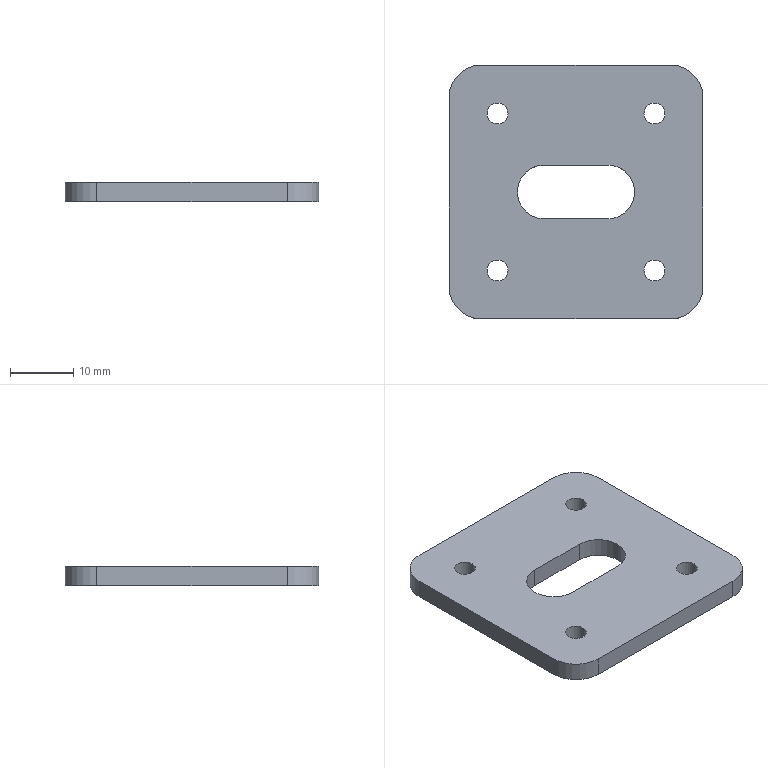Part | SolidWorks | features BaseBody 1 | 1 solid | 23 faces | box 40 x 40 x 3 mm | volume 4208 mm3 | cylinder 15 | plane 8 | commonest cylinder face diameters 3.3 x8 10 x4 8.5 x3
STEP:
#1=CARTESIAN_POINT('',(30.725,-32.375,0.));
#2=VERTEX_POINT('',#1);
#3=CARTESIAN_POINT('',(30.725,-32.375,3.));
#4=VERTEX_POINT('',#3);
#5=CARTESIAN_POINT('',(30.725,-32.375,3.));
#6=DIRECTION('',(0.,0.,1.));
#7=VECTOR('',#6,1000.);
#8=LINE('',#5,#7);
#9=EDGE_CURVE('',#2,#4,#8,.T.);
#10=ORIENTED_EDGE('',*,*,#9,.F.);
#11=CARTESIAN_POINT('',(34.025,-32.375,0.));
#12=VERTEX_POINT('',#11);
#13=CARTESIAN_POINT('',(32.375,-32.375,0.));
#14=DIRECTION('',(0.,0.,1.));
#15=DIRECTION('',(1.,0.,0.));
#16=AXIS2_PLACEMENT_3D('',#13,#14,#15);
#17=CIRCLE('',#16,1.65);
#18=EDGE_CURVE('',#12,#2,#17,.T.);
#19=ORIENTED_EDGE('',*,*,#18,.F.);
#20=CARTESIAN_POINT('',(34.025,-32.375,3.));
#21=VERTEX_POINT('',#20);
#22=CARTESIAN_POINT('',(34.025,-32.375,3.));
#23=DIRECTION('',(0.,0.,1.));
#24=VECTOR('',#23,1000.);
#25=LINE('',#22,#24);
#26=EDGE_CURVE('',#12,#21,#25,.T.);
#27=ORIENTED_EDGE('',*,*,#26,.T.);
#28=CARTESIAN_POINT('',(32.375,-32.375,3.));
#29=DIRECTION('',(0.,0.,1.));
#30=DIRECTION('',(1.,0.,0.));
#31=AXIS2_PLACEMENT_3D('',#28,#29,#30);
#32=CIRCLE('',#31,1.65);
#33=EDGE_CURVE('',#21,#4,#32,.T.);
#34=ORIENTED_EDGE('',*,*,#33,.T.);
#35=EDGE_LOOP('',(#10,#19,#27,#34));
#36=FACE_OUTER_BOUND('',#35,.T.);
#37=CARTESIAN_POINT('',(32.375,-32.375,3.));
#38=DIRECTION('',(0.,0.,1.));
#39=DIRECTION('',(1.,0.,0.));
#40=AXIS2_PLACEMENT_3D('',#37,#38,#39);
#41=CYLINDRICAL_SURFACE('',#40,1.65);
#42=ADVANCED_FACE('',(#36),#41,.F.);
#43=CARTESIAN_POINT('',(5.975,-32.375,0.));
#44=VERTEX_POINT('',#43);
#45=CARTESIAN_POINT('',(5.975,-32.375,3.));
#46=VERTEX_POINT('',#45);
#47=CARTESIAN_POINT('',(5.975,-32.375,3.));
#48=DIRECTION('',(0.,0.,1.));
#49=VECTOR('',#48,1000.);
#50=LINE('',#47,#49);
#51=EDGE_CURVE('',#44,#46,#50,.T.);
#52=ORIENTED_EDGE('',*,*,#51,.F.);
#53=CARTESIAN_POINT('',(9.275,-32.375,0.));
#54=VERTEX_POINT('',#53);
#55=CARTESIAN_POINT('',(7.625,-32.375,0.));
#56=DIRECTION('',(0.,0.,1.));
#57=DIRECTION('',(1.,0.,0.));
#58=AXIS2_PLACEMENT_3D('',#55,#56,#57);
#59=CIRCLE('',#58,1.65);
#60=EDGE_CURVE('',#54,#44,#59,.T.);
#61=ORIENTED_EDGE('',*,*,#60,.F.);
#62=CARTESIAN_POINT('',(9.275,-32.375,3.));
#63=VERTEX_POINT('',#62);
#64=CARTESIAN_POINT('',(9.275,-32.375,3.));
#65=DIRECTION('',(0.,0.,1.));
#66=VECTOR('',#65,1000.);
#67=LINE('',#64,#66);
#68=EDGE_CURVE('',#54,#63,#67,.T.);
#69=ORIENTED_EDGE('',*,*,#68,.T.);
#70=CARTESIAN_POINT('',(7.625,-32.375,3.));
#71=DIRECTION('',(0.,0.,1.));
#72=DIRECTION('',(1.,0.,0.));
#73=AXIS2_PLACEMENT_3D('',#70,#71,#72);
#74=CIRCLE('',#73,1.65);
#75=EDGE_CURVE('',#63,#46,#74,.T.);
#76=ORIENTED_EDGE('',*,*,#75,.T.);
#77=EDGE_LOOP('',(#52,#61,#69,#76));
#78=FACE_OUTER_BOUND('',#77,.T.);
#79=CARTESIAN_POINT('',(7.625,-32.375,3.));
#80=DIRECTION('',(0.,0.,1.));
#81=DIRECTION('',(1.,0.,0.));
#82=AXIS2_PLACEMENT_3D('',#79,#80,#81);
#83=CYLINDRICAL_SURFACE('',#82,1.65);
#84=ADVANCED_FACE('',(#78),#83,.F.);
#85=CARTESIAN_POINT('',(30.725,-7.625,0.));
#86=VERTEX_POINT('',#85);
#87=CARTESIAN_POINT('',(30.725,-7.625,3.));
#88=VERTEX_POINT('',#87);
#89=CARTESIAN_POINT('',(30.725,-7.625,3.));
#90=DIRECTION('',(0.,0.,1.));
#91=VECTOR('',#90,1000.);
#92=LINE('',#89,#91);
#93=EDGE_CURVE('',#86,#88,#92,.T.);
#94=ORIENTED_EDGE('',*,*,#93,.F.);
#95=CARTESIAN_POINT('',(34.025,-7.625,0.));
#96=VERTEX_POINT('',#95);
#97=CARTESIAN_POINT('',(32.375,-7.625,0.));
#98=DIRECTION('',(0.,0.,1.));
#99=DIRECTION('',(1.,0.,0.));
#100=AXIS2_PLACEMENT_3D('',#97,#98,#99);
#101=CIRCLE('',#100,1.65);
#102=EDGE_CURVE('',#96,#86,#101,.T.);
#103=ORIENTED_EDGE('',*,*,#102,.F.);
#104=CARTESIAN_POINT('',(34.025,-7.625,3.));
#105=VERTEX_POINT('',#104);
#106=CARTESIAN_POINT('',(34.025,-7.625,3.));
#107=DIRECTION('',(0.,0.,1.));
#108=VECTOR('',#107,1000.);
#109=LINE('',#106,#108);
#110=EDGE_CURVE('',#96,#105,#109,.T.);
#111=ORIENTED_EDGE('',*,*,#110,.T.);
#112=CARTESIAN_POINT('',(32.375,-7.625,3.));
#113=DIRECTION('',(0.,0.,1.));
#114=DIRECTION('',(1.,0.,0.));
#115=AXIS2_PLACEMENT_3D('',#112,#113,#114);
#116=CIRCLE('',#115,1.65);
#117=EDGE_CURVE('',#105,#88,#116,.T.);
#118=ORIENTED_EDGE('',*,*,#117,.T.);
#119=EDGE_LOOP('',(#94,#103,#111,#118));
#120=FACE_OUTER_BOUND('',#119,.T.);
#121=CARTESIAN_POINT('',(32.375,-7.625,3.));
#122=DIRECTION('',(0.,0.,1.));
#123=DIRECTION('',(1.,0.,0.));
#124=AXIS2_PLACEMENT_3D('',#121,#122,#123);
#125=CYLINDRICAL_SURFACE('',#124,1.65);
#126=ADVANCED_FACE('',(#120),#125,.F.);
#127=CARTESIAN_POINT('',(5.975,-7.625,0.));
#128=VERTEX_POINT('',#127);
#129=CARTESIAN_POINT('',(5.975,-7.625,3.));
#130=VERTEX_POINT('',#129);
#131=CARTESIAN_POINT('',(5.975,-7.625,3.));
#132=DIRECTION('',(0.,0.,1.));
#133=VECTOR('',#132,1000.);
#134=LINE('',#131,#133);
#135=EDGE_CURVE('',#128,#130,#134,.T.);
#136=ORIENTED_EDGE('',*,*,#135,.F.);
#137=CARTESIAN_POINT('',(9.275,-7.625,0.));
#138=VERTEX_POINT('',#137);
#139=CARTESIAN_POINT('',(7.625,-7.625,0.));
#140=DIRECTION('',(0.,0.,1.));
#141=DIRECTION('',(1.,0.,0.));
#142=AXIS2_PLACEMENT_3D('',#139,#140,#141);
#143=CIRCLE('',#142,1.65);
#144=EDGE_CURVE('',#138,#128,#143,.T.);
#145=ORIENTED_EDGE('',*,*,#144,.F.);
#146=CARTESIAN_POINT('',(9.275,-7.625,3.));
#147=VERTEX_POINT('',#146);
#148=CARTESIAN_POINT('',(9.275,-7.625,3.));
#149=DIRECTION('',(0.,0.,1.));
#150=VECTOR('',#149,1000.);
#151=LINE('',#148,#150);
#152=EDGE_CURVE('',#138,#147,#151,.T.);
#153=ORIENTED_EDGE('',*,*,#152,.T.);
#154=CARTESIAN_POINT('',(7.625,-7.625,3.));
#155=DIRECTION('',(0.,0.,1.));
#156=DIRECTION('',(1.,0.,0.));
#157=AXIS2_PLACEMENT_3D('',#154,#155,#156);
#158=CIRCLE('',#157,1.65);
#159=EDGE_CURVE('',#147,#130,#158,.T.);
#160=ORIENTED_EDGE('',*,*,#159,.T.);
#161=EDGE_LOOP('',(#136,#145,#153,#160));
#162=FACE_OUTER_BOUND('',#161,.T.);
#163=CARTESIAN_POINT('',(7.625,-7.625,3.));
#164=DIRECTION('',(0.,0.,1.));
#165=DIRECTION('',(1.,0.,0.));
#166=AXIS2_PLACEMENT_3D('',#163,#164,#165);
#167=CYLINDRICAL_SURFACE('',#166,1.65);
#168=ADVANCED_FACE('',(#162),#167,.F.);
#169=CARTESIAN_POINT('',(15.,-15.75,0.));
#170=VERTEX_POINT('',#169);
#171=CARTESIAN_POINT('',(15.,-15.75,3.));
#172=VERTEX_POINT('',#171);
#173=CARTESIAN_POINT('',(15.,-15.75,-20.359));
#174=DIRECTION('',(0.,0.,1.));
#175=VECTOR('',#174,1000.);
#176=LINE('',#173,#175);
#177=EDGE_CURVE('',#170,#172,#176,.T.);
#178=ORIENTED_EDGE('',*,*,#177,.T.);
#179=CARTESIAN_POINT('',(15.,-24.25,3.));
#180=VERTEX_POINT('',#179);
#181=CARTESIAN_POINT('',(15.,-20.,3.));
#182=DIRECTION('',(0.,0.,1.));
#183=DIRECTION('',(1.,0.,0.));
#184=AXIS2_PLACEMENT_3D('',#181,#182,#183);
#185=CIRCLE('',#184,4.25);
#186=EDGE_CURVE('',#172,#180,#185,.T.);
#187=ORIENTED_EDGE('',*,*,#186,.T.);
#188=CARTESIAN_POINT('',(15.,-24.25,0.));
#189=VERTEX_POINT('',#188);
#190=CARTESIAN_POINT('',(15.,-24.25,-20.359));
#191=DIRECTION('',(0.,0.,1.));
#192=VECTOR('',#191,1000.);
#193=LINE('',#190,#192);
#194=EDGE_CURVE('',#189,#180,#193,.T.);
#195=ORIENTED_EDGE('',*,*,#194,.F.);
#196=CARTESIAN_POINT('',(15.,-20.,0.));
#197=DIRECTION('',(0.,0.,1.));
#198=DIRECTION('',(-1.,0.,0.));
#199=AXIS2_PLACEMENT_3D('',#196,#197,#198);
#200=CIRCLE('',#199,4.25);
#201=EDGE_CURVE('',#170,#189,#200,.T.);
#202=ORIENTED_EDGE('',*,*,#201,.F.);
#203=EDGE_LOOP('',(#178,#187,#195,#202));
#204=FACE_OUTER_BOUND('',#203,.T.);
#205=CARTESIAN_POINT('',(15.,-20.,-20.359));
#206=DIRECTION('',(0.,0.,1.));
#207=DIRECTION('',(1.,0.,0.));
#208=AXIS2_PLACEMENT_3D('',#205,#206,#207);
#209=CYLINDRICAL_SURFACE('',#208,4.25);
#210=ADVANCED_FACE('',(#204),#209,.F.);
#211=CARTESIAN_POINT('',(25.,-15.75,0.));
#212=VERTEX_POINT('',#211);
#213=CARTESIAN_POINT('',(25.,-15.75,3.));
#214=VERTEX_POINT('',#213);
#215=CARTESIAN_POINT('',(25.,-15.75,-20.359));
#216=DIRECTION('',(0.,0.,1.));
#217=VECTOR('',#216,1000.);
#218=LINE('',#215,#217);
#219=EDGE_CURVE('',#212,#214,#218,.T.);
#220=ORIENTED_EDGE('',*,*,#219,.T.);
#221=CARTESIAN_POINT('',(15.,-15.75,3.));
#222=DIRECTION('',(-1.,0.,0.));
#223=VECTOR('',#222,1000.);
#224=LINE('',#221,#223);
#225=EDGE_CURVE('',#214,#172,#224,.T.);
#226=ORIENTED_EDGE('',*,*,#225,.T.);
#227=ORIENTED_EDGE('',*,*,#177,.F.);
#228=CARTESIAN_POINT('',(15.,-15.75,0.));
#229=DIRECTION('',(-1.,0.,0.));
#230=VECTOR('',#229,1000.);
#231=LINE('',#228,#230);
#232=EDGE_CURVE('',#212,#170,#231,.T.);
#233=ORIENTED_EDGE('',*,*,#232,.F.);
#234=EDGE_LOOP('',(#220,#226,#227,#233));
#235=FACE_OUTER_BOUND('',#234,.T.);
#236=CARTESIAN_POINT('',(15.,-15.75,-20.359));
#237=DIRECTION('',(0.,1.,0.));
#238=DIRECTION('',(1.,0.,0.));
#239=AXIS2_PLACEMENT_3D('',#236,#237,#238);
#240=PLANE('',#239);
#241=ADVANCED_FACE('',(#235),#240,.F.);
#242=CARTESIAN_POINT('',(29.25,-20.,0.));
#243=VERTEX_POINT('',#242);
#244=CARTESIAN_POINT('',(29.25,-20.,3.));
#245=VERTEX_POINT('',#244);
#246=CARTESIAN_POINT('',(29.25,-20.,-20.359));
#247=DIRECTION('',(0.,0.,1.));
#248=VECTOR('',#247,1000.);
#249=LINE('',#246,#248);
#250=EDGE_CURVE('',#243,#245,#249,.T.);
#251=ORIENTED_EDGE('',*,*,#250,.F.);
#252=CARTESIAN_POINT('',(25.,-24.25,0.));
#253=VERTEX_POINT('',#252);
#254=CARTESIAN_POINT('',(25.,-20.,0.));
#255=DIRECTION('',(0.,0.,1.));
#256=DIRECTION('',(-1.,0.,0.));
#257=AXIS2_PLACEMENT_3D('',#254,#255,#256);
#258=CIRCLE('',#257,4.25);
#259=EDGE_CURVE('',#253,#243,#258,.T.);
#260=ORIENTED_EDGE('',*,*,#259,.F.);
#261=CARTESIAN_POINT('',(25.,-24.25,3.));
#262=VERTEX_POINT('',#261);
#263=CARTESIAN_POINT('',(25.,-24.25,-20.359));
#264=DIRECTION('',(0.,0.,1.));
#265=VECTOR('',#264,1000.);
#266=LINE('',#263,#265);
#267=EDGE_CURVE('',#253,#262,#266,.T.);
#268=ORIENTED_EDGE('',*,*,#267,.T.);
#269=CARTESIAN_POINT('',(25.,-20.,3.));
#270=DIRECTION('',(0.,0.,1.));
#271=DIRECTION('',(1.,0.,0.));
#272=AXIS2_PLACEMENT_3D('',#269,#270,#271);
#273=CIRCLE('',#272,4.25);
#274=EDGE_CURVE('',#262,#245,#273,.T.);
#275=ORIENTED_EDGE('',*,*,#274,.T.);
#276=EDGE_LOOP('',(#251,#260,#268,#275));
#277=FACE_OUTER_BOUND('',#276,.T.);
#278=CARTESIAN_POINT('',(25.,-20.,-20.359));
#279=DIRECTION('',(0.,0.,1.));
#280=DIRECTION('',(1.,0.,0.));
#281=AXIS2_PLACEMENT_3D('',#278,#279,#280);
#282=CYLINDRICAL_SURFACE('',#281,4.25);
#283=ADVANCED_FACE('',(#277),#282,.F.);
#284=ORIENTED_EDGE('',*,*,#194,.T.);
#285=CARTESIAN_POINT('',(15.,-24.25,3.));
#286=DIRECTION('',(1.,0.,0.));
#287=VECTOR('',#286,1000.);
#288=LINE('',#285,#287);
#289=EDGE_CURVE('',#180,#262,#288,.T.);
#290=ORIENTED_EDGE('',*,*,#289,.T.);
#291=ORIENTED_EDGE('',*,*,#267,.F.);
#292=CARTESIAN_POINT('',(15.,-24.25,0.));
#293=DIRECTION('',(1.,0.,0.));
#294=VECTOR('',#293,1000.);
#295=LINE('',#292,#294);
#296=EDGE_CURVE('',#189,#253,#295,.T.);
#297=ORIENTED_EDGE('',*,*,#296,.F.);
#298=EDGE_LOOP('',(#284,#290,#291,#297));
#299=FACE_OUTER_BOUND('',#298,.T.);
#300=CARTESIAN_POINT('',(15.,-24.25,-20.359));
#301=DIRECTION('',(0.,-1.,0.));
#302=DIRECTION('',(0.,0.,-1.));
#303=AXIS2_PLACEMENT_3D('',#300,#301,#302);
#304=PLANE('',#303);
#305=ADVANCED_FACE('',(#299),#304,.F.);
#306=CARTESIAN_POINT('',(5.,0.,3.));
#307=VERTEX_POINT('',#306);
#308=CARTESIAN_POINT('',(0.,-5.,3.));
#309=VERTEX_POINT('',#308);
#310=CARTESIAN_POINT('',(5.,-5.,3.));
#311=DIRECTION('',(0.,0.,1.));
#312=DIRECTION('',(-1.,0.,0.));
#313=AXIS2_PLACEMENT_3D('',#310,#311,#312);
#314=CIRCLE('',#313,5.);
#315=EDGE_CURVE('',#307,#309,#314,.T.);
#316=ORIENTED_EDGE('',*,*,#315,.F.);
#317=CARTESIAN_POINT('',(5.,0.,0.));
#318=VERTEX_POINT('',#317);
#319=CARTESIAN_POINT('',(5.,0.,3.));
#320=DIRECTION('',(0.,0.,1.));
#321=VECTOR('',#320,1000.);
#322=LINE('',#319,#321);
#323=EDGE_CURVE('',#318,#307,#322,.T.);
#324=ORIENTED_EDGE('',*,*,#323,.F.);
#325=CARTESIAN_POINT('',(0.,-5.,0.));
#326=VERTEX_POINT('',#325);
#327=CARTESIAN_POINT('',(5.,-5.,0.));
#328=DIRECTION('',(0.,0.,-1.));
#329=DIRECTION('',(-1.,0.,0.));
#330=AXIS2_PLACEMENT_3D('',#327,#328,#329);
#331=CIRCLE('',#330,5.);
#332=EDGE_CURVE('',#326,#318,#331,.T.);
#333=ORIENTED_EDGE('',*,*,#332,.F.);
#334=CARTESIAN_POINT('',(0.,-5.,3.));
#335=DIRECTION('',(0.,0.,-1.));
#336=VECTOR('',#335,1000.);
#337=LINE('',#334,#336);
#338=EDGE_CURVE('',#309,#326,#337,.T.);
#339=ORIENTED_EDGE('',*,*,#338,.F.);
#340=EDGE_LOOP('',(#316,#324,#333,#339));
#341=FACE_OUTER_BOUND('',#340,.T.);
#342=CARTESIAN_POINT('',(5.,-5.,3.));
#343=DIRECTION('',(0.,0.,-1.));
#344=DIRECTION('',(-1.,0.,0.));
#345=AXIS2_PLACEMENT_3D('',#342,#343,#344);
#346=CYLINDRICAL_SURFACE('',#345,5.);
#347=ADVANCED_FACE('',(#341),#346,.T.);
#348=CARTESIAN_POINT('',(0.,-35.,3.));
#349=VERTEX_POINT('',#348);
#350=CARTESIAN_POINT('',(5.,-40.,3.));
#351=VERTEX_POINT('',#350);
#352=CARTESIAN_POINT('',(5.,-35.,3.));
#353=DIRECTION('',(0.,0.,1.));
#354=DIRECTION('',(-1.,0.,0.));
#355=AXIS2_PLACEMENT_3D('',#352,#353,#354);
#356=CIRCLE('',#355,5.);
#357=EDGE_CURVE('',#349,#351,#356,.T.);
#358=ORIENTED_EDGE('',*,*,#357,.F.);
#359=CARTESIAN_POINT('',(0.,-35.,0.));
#360=VERTEX_POINT('',#359);
#361=CARTESIAN_POINT('',(0.,-35.,3.));
#362=DIRECTION('',(0.,0.,1.));
#363=VECTOR('',#362,1000.);
#364=LINE('',#361,#363);
#365=EDGE_CURVE('',#360,#349,#364,.T.);
#366=ORIENTED_EDGE('',*,*,#365,.F.);
#367=CARTESIAN_POINT('',(5.,-40.,0.));
#368=VERTEX_POINT('',#367);
#369=CARTESIAN_POINT('',(5.,-35.,0.));
#370=DIRECTION('',(0.,0.,-1.));
#371=DIRECTION('',(-1.,0.,0.));
#372=AXIS2_PLACEMENT_3D('',#369,#370,#371);
#373=CIRCLE('',#372,5.);
#374=EDGE_CURVE('',#368,#360,#373,.T.);
#375=ORIENTED_EDGE('',*,*,#374,.F.);
#376=CARTESIAN_POINT('',(5.,-40.,3.));
#377=DIRECTION('',(0.,0.,-1.));
#378=VECTOR('',#377,1000.);
#379=LINE('',#376,#378);
#380=EDGE_CURVE('',#351,#368,#379,.T.);
#381=ORIENTED_EDGE('',*,*,#380,.F.);
#382=EDGE_LOOP('',(#358,#366,#375,#381));
#383=FACE_OUTER_BOUND('',#382,.T.);
#384=CARTESIAN_POINT('',(5.,-35.,3.));
#385=DIRECTION('',(0.,0.,-1.));
#386=DIRECTION('',(-1.,0.,0.));
#387=AXIS2_PLACEMENT_3D('',#384,#385,#386);
#388=CYLINDRICAL_SURFACE('',#387,5.);
#389=ADVANCED_FACE('',(#383),#388,.T.);
#390=CARTESIAN_POINT('',(35.,-40.,3.));
#391=VERTEX_POINT('',#390);
#392=CARTESIAN_POINT('',(40.,-35.,3.));
#393=VERTEX_POINT('',#392);
#394=CARTESIAN_POINT('',(35.,-35.,3.));
#395=DIRECTION('',(0.,0.,1.));
#396=DIRECTION('',(-1.,0.,0.));
#397=AXIS2_PLACEMENT_3D('',#394,#395,#396);
#398=CIRCLE('',#397,5.);
#399=EDGE_CURVE('',#391,#393,#398,.T.);
#400=ORIENTED_EDGE('',*,*,#399,.F.);
#401=CARTESIAN_POINT('',(35.,-40.,0.));
#402=VERTEX_POINT('',#401);
#403=CARTESIAN_POINT('',(35.,-40.,3.));
#404=DIRECTION('',(0.,0.,1.));
#405=VECTOR('',#404,1000.);
#406=LINE('',#403,#405);
#407=EDGE_CURVE('',#402,#391,#406,.T.);
#408=ORIENTED_EDGE('',*,*,#407,.F.);
#409=CARTESIAN_POINT('',(40.,-35.,0.));
#410=VERTEX_POINT('',#409);
#411=CARTESIAN_POINT('',(35.,-35.,0.));
#412=DIRECTION('',(0.,0.,-1.));
#413=DIRECTION('',(-1.,0.,0.));
#414=AXIS2_PLACEMENT_3D('',#411,#412,#413);
#415=CIRCLE('',#414,5.);
#416=EDGE_CURVE('',#410,#402,#415,.T.);
#417=ORIENTED_EDGE('',*,*,#416,.F.);
#418=CARTESIAN_POINT('',(40.,-35.,3.));
#419=DIRECTION('',(0.,0.,-1.));
#420=VECTOR('',#419,1000.);
#421=LINE('',#418,#420);
#422=EDGE_CURVE('',#393,#410,#421,.T.);
#423=ORIENTED_EDGE('',*,*,#422,.F.);
#424=EDGE_LOOP('',(#400,#408,#417,#423));
#425=FACE_OUTER_BOUND('',#424,.T.);
#426=CARTESIAN_POINT('',(35.,-35.,3.));
#427=DIRECTION('',(0.,0.,-1.));
#428=DIRECTION('',(-1.,0.,0.));
#429=AXIS2_PLACEMENT_3D('',#426,#427,#428);
#430=CYLINDRICAL_SURFACE('',#429,5.);
#431=ADVANCED_FACE('',(#425),#430,.T.);
#432=CARTESIAN_POINT('',(40.,-5.,3.));
#433=VERTEX_POINT('',#432);
#434=CARTESIAN_POINT('',(35.,0.,3.));
#435=VERTEX_POINT('',#434);
#436=CARTESIAN_POINT('',(35.,-5.,3.));
#437=DIRECTION('',(0.,0.,1.));
#438=DIRECTION('',(-1.,0.,0.));
#439=AXIS2_PLACEMENT_3D('',#436,#437,#438);
#440=CIRCLE('',#439,5.);
#441=EDGE_CURVE('',#433,#435,#440,.T.);
#442=ORIENTED_EDGE('',*,*,#441,.F.);
#443=CARTESIAN_POINT('',(40.,-5.,0.));
#444=VERTEX_POINT('',#443);
#445=CARTESIAN_POINT('',(40.,-5.,3.));
#446=DIRECTION('',(0.,0.,1.));
#447=VECTOR('',#446,1000.);
#448=LINE('',#445,#447);
#449=EDGE_CURVE('',#444,#433,#448,.T.);
#450=ORIENTED_EDGE('',*,*,#449,.F.);
#451=CARTESIAN_POINT('',(35.,0.,0.));
#452=VERTEX_POINT('',#451);
#453=CARTESIAN_POINT('',(35.,-5.,0.));
#454=DIRECTION('',(0.,0.,-1.));
#455=DIRECTION('',(-1.,0.,0.));
#456=AXIS2_PLACEMENT_3D('',#453,#454,#455);
#457=CIRCLE('',#456,5.);
#458=EDGE_CURVE('',#452,#444,#457,.T.);
#459=ORIENTED_EDGE('',*,*,#458,.F.);
#460=CARTESIAN_POINT('',(35.,0.,3.));
#461=DIRECTION('',(0.,0.,-1.));
#462=VECTOR('',#461,1000.);
#463=LINE('',#460,#462);
#464=EDGE_CURVE('',#435,#452,#463,.T.);
#465=ORIENTED_EDGE('',*,*,#464,.F.);
#466=EDGE_LOOP('',(#442,#450,#459,#465));
#467=FACE_OUTER_BOUND('',#466,.T.);
#468=CARTESIAN_POINT('',(35.,-5.,3.));
#469=DIRECTION('',(0.,0.,-1.));
#470=DIRECTION('',(-1.,0.,0.));
#471=AXIS2_PLACEMENT_3D('',#468,#469,#470);
#472=CYLINDRICAL_SURFACE('',#471,5.);
#473=ADVANCED_FACE('',(#467),#472,.T.);
#474=ORIENTED_EDGE('',*,*,#274,.F.);
#475=ORIENTED_EDGE('',*,*,#289,.F.);
#476=ORIENTED_EDGE('',*,*,#186,.F.);
#477=ORIENTED_EDGE('',*,*,#225,.F.);
#478=CARTESIAN_POINT('',(25.,-20.,3.));
#479=DIRECTION('',(0.,0.,1.));
#480=DIRECTION('',(1.,0.,0.));
#481=AXIS2_PLACEMENT_3D('',#478,#479,#480);
#482=CIRCLE('',#481,4.25);
#483=EDGE_CURVE('',#245,#214,#482,.T.);
#484=ORIENTED_EDGE('',*,*,#483,.F.);
#485=EDGE_LOOP('',(#474,#475,#476,#477,#484));
#486=FACE_BOUND('',#485,.T.);
#487=ORIENTED_EDGE('',*,*,#159,.F.);
#488=CARTESIAN_POINT('',(7.625,-7.625,3.));
#489=DIRECTION('',(0.,0.,1.));
#490=DIRECTION('',(1.,0.,0.));
#491=AXIS2_PLACEMENT_3D('',#488,#489,#490);
#492=CIRCLE('',#491,1.65);
#493=EDGE_CURVE('',#130,#147,#492,.T.);
#494=ORIENTED_EDGE('',*,*,#493,.F.);
#495=EDGE_LOOP('',(#487,#494));
#496=FACE_BOUND('',#495,.T.);
#497=ORIENTED_EDGE('',*,*,#117,.F.);
#498=CARTESIAN_POINT('',(32.375,-7.625,3.));
#499=DIRECTION('',(0.,0.,1.));
#500=DIRECTION('',(1.,0.,0.));
#501=AXIS2_PLACEMENT_3D('',#498,#499,#500);
#502=CIRCLE('',#501,1.65);
#503=EDGE_CURVE('',#88,#105,#502,.T.);
#504=ORIENTED_EDGE('',*,*,#503,.F.);
#505=EDGE_LOOP('',(#497,#504));
#506=FACE_BOUND('',#505,.T.);
#507=ORIENTED_EDGE('',*,*,#75,.F.);
#508=CARTESIAN_POINT('',(7.625,-32.375,3.));
#509=DIRECTION('',(0.,0.,1.));
#510=DIRECTION('',(1.,0.,0.));
#511=AXIS2_PLACEMENT_3D('',#508,#509,#510);
#512=CIRCLE('',#511,1.65);
#513=EDGE_CURVE('',#46,#63,#512,.T.);
#514=ORIENTED_EDGE('',*,*,#513,.F.);
#515=EDGE_LOOP('',(#507,#514));
#516=FACE_BOUND('',#515,.T.);
#517=ORIENTED_EDGE('',*,*,#33,.F.);
#518=CARTESIAN_POINT('',(32.375,-32.375,3.));
#519=DIRECTION('',(0.,0.,1.));
#520=DIRECTION('',(1.,0.,0.));
#521=AXIS2_PLACEMENT_3D('',#518,#519,#520);
#522=CIRCLE('',#521,1.65);
#523=EDGE_CURVE('',#4,#21,#522,.T.);
#524=ORIENTED_EDGE('',*,*,#523,.F.);
#525=EDGE_LOOP('',(#517,#524));
#526=FACE_BOUND('',#525,.T.);
#527=CARTESIAN_POINT('',(40.,-40.,3.));
#528=DIRECTION('',(0.,1.,0.));
#529=VECTOR('',#528,1000.);
#530=LINE('',#527,#529);
#531=EDGE_CURVE('',#393,#433,#530,.T.);
#532=ORIENTED_EDGE('',*,*,#531,.T.);
#533=ORIENTED_EDGE('',*,*,#441,.T.);
#534=CARTESIAN_POINT('',(0.,0.,3.));
#535=DIRECTION('',(-1.,0.,0.));
#536=VECTOR('',#535,1000.);
#537=LINE('',#534,#536);
#538=EDGE_CURVE('',#435,#307,#537,.T.);
#539=ORIENTED_EDGE('',*,*,#538,.T.);
#540=ORIENTED_EDGE('',*,*,#315,.T.);
#541=CARTESIAN_POINT('',(0.,-40.,3.));
#542=DIRECTION('',(0.,-1.,0.));
#543=VECTOR('',#542,1000.);
#544=LINE('',#541,#543);
#545=EDGE_CURVE('',#309,#349,#544,.T.);
#546=ORIENTED_EDGE('',*,*,#545,.T.);
#547=ORIENTED_EDGE('',*,*,#357,.T.);
#548=CARTESIAN_POINT('',(0.,-40.,3.));
#549=DIRECTION('',(1.,0.,0.));
#550=VECTOR('',#549,1000.);
#551=LINE('',#548,#550);
#552=EDGE_CURVE('',#351,#391,#551,.T.);
#553=ORIENTED_EDGE('',*,*,#552,.T.);
#554=ORIENTED_EDGE('',*,*,#399,.T.);
#555=EDGE_LOOP('',(#532,#533,#539,#540,#546,#547,#553,#554));
#556=FACE_OUTER_BOUND('',#555,.T.);
#557=CARTESIAN_POINT('',(0.,0.,3.));
#558=DIRECTION('',(0.,0.,-1.));
#559=DIRECTION('',(0.,-1.,0.));
#560=AXIS2_PLACEMENT_3D('',#557,#558,#559);
#561=PLANE('',#560);
#562=ADVANCED_FACE('',(#486,#496,#506,#516,#526,#556),#561,.F.);
#563=CARTESIAN_POINT('',(0.,-40.,0.));
#564=DIRECTION('',(1.,0.,0.));
#565=VECTOR('',#564,1000.);
#566=LINE('',#563,#565);
#567=EDGE_CURVE('',#368,#402,#566,.T.);
#568=ORIENTED_EDGE('',*,*,#567,.T.);
#569=ORIENTED_EDGE('',*,*,#407,.T.);
#570=ORIENTED_EDGE('',*,*,#552,.F.);
#571=ORIENTED_EDGE('',*,*,#380,.T.);
#572=EDGE_LOOP('',(#568,#569,#570,#571));
#573=FACE_OUTER_BOUND('',#572,.T.);
#574=CARTESIAN_POINT('',(0.,-40.,3.));
#575=DIRECTION('',(0.,1.,0.));
#576=DIRECTION('',(1.,0.,0.));
#577=AXIS2_PLACEMENT_3D('',#574,#575,#576);
#578=PLANE('',#577);
#579=ADVANCED_FACE('',(#573),#578,.F.);
#580=CARTESIAN_POINT('',(0.,-40.,0.));
#581=DIRECTION('',(0.,-1.,0.));
#582=VECTOR('',#581,1000.);
#583=LINE('',#580,#582);
#584=EDGE_CURVE('',#326,#360,#583,.T.);
#585=ORIENTED_EDGE('',*,*,#584,.T.);
#586=ORIENTED_EDGE('',*,*,#365,.T.);
#587=ORIENTED_EDGE('',*,*,#545,.F.);
#588=ORIENTED_EDGE('',*,*,#338,.T.);
#589=EDGE_LOOP('',(#585,#586,#587,#588));
#590=FACE_OUTER_BOUND('',#589,.T.);
#591=CARTESIAN_POINT('',(0.,-40.,3.));
#592=DIRECTION('',(1.,0.,0.));
#593=DIRECTION('',(0.,1.,0.));
#594=AXIS2_PLACEMENT_3D('',#591,#592,#593);
#595=PLANE('',#594);
#596=ADVANCED_FACE('',(#590),#595,.F.);
#597=ORIENTED_EDGE('',*,*,#538,.F.);
#598=ORIENTED_EDGE('',*,*,#464,.T.);
#599=CARTESIAN_POINT('',(0.,0.,0.));
#600=DIRECTION('',(-1.,0.,0.));
#601=VECTOR('',#600,1000.);
#602=LINE('',#599,#601);
#603=EDGE_CURVE('',#452,#318,#602,.T.);
#604=ORIENTED_EDGE('',*,*,#603,.T.);
#605=ORIENTED_EDGE('',*,*,#323,.T.);
#606=EDGE_LOOP('',(#597,#598,#604,#605));
#607=FACE_OUTER_BOUND('',#606,.T.);
#608=CARTESIAN_POINT('',(0.,0.,3.));
#609=DIRECTION('',(0.,-1.,0.));
#610=DIRECTION('',(0.,0.,-1.));
#611=AXIS2_PLACEMENT_3D('',#608,#609,#610);
#612=PLANE('',#611);
#613=ADVANCED_FACE('',(#607),#612,.F.);
#614=CARTESIAN_POINT('',(40.,-40.,0.));
#615=DIRECTION('',(0.,1.,0.));
#616=VECTOR('',#615,1000.);
#617=LINE('',#614,#616);
#618=EDGE_CURVE('',#410,#444,#617,.T.);
#619=ORIENTED_EDGE('',*,*,#618,.T.);
#620=ORIENTED_EDGE('',*,*,#449,.T.);
#621=ORIENTED_EDGE('',*,*,#531,.F.);
#622=ORIENTED_EDGE('',*,*,#422,.T.);
#623=EDGE_LOOP('',(#619,#620,#621,#622));
#624=FACE_OUTER_BOUND('',#623,.T.);
#625=CARTESIAN_POINT('',(40.,-40.,3.));
#626=DIRECTION('',(-1.,0.,0.));
#627=DIRECTION('',(0.,0.,1.));
#628=AXIS2_PLACEMENT_3D('',#625,#626,#627);
#629=PLANE('',#628);
#630=ADVANCED_FACE('',(#624),#629,.F.);
#631=ORIENTED_EDGE('',*,*,#144,.T.);
#632=CARTESIAN_POINT('',(7.625,-7.625,0.));
#633=DIRECTION('',(0.,0.,1.));
#634=DIRECTION('',(1.,0.,0.));
#635=AXIS2_PLACEMENT_3D('',#632,#633,#634);
#636=CIRCLE('',#635,1.65);
#637=EDGE_CURVE('',#128,#138,#636,.T.);
#638=ORIENTED_EDGE('',*,*,#637,.T.);
#639=EDGE_LOOP('',(#631,#638));
#640=FACE_BOUND('',#639,.T.);
#641=ORIENTED_EDGE('',*,*,#296,.T.);
#642=ORIENTED_EDGE('',*,*,#259,.T.);
#643=CARTESIAN_POINT('',(25.,-20.,0.));
#644=DIRECTION('',(0.,0.,1.));
#645=DIRECTION('',(-1.,0.,0.));
#646=AXIS2_PLACEMENT_3D('',#643,#644,#645);
#647=CIRCLE('',#646,4.25);
#648=EDGE_CURVE('',#243,#212,#647,.T.);
#649=ORIENTED_EDGE('',*,*,#648,.T.);
#650=ORIENTED_EDGE('',*,*,#232,.T.);
#651=ORIENTED_EDGE('',*,*,#201,.T.);
#652=EDGE_LOOP('',(#641,#642,#649,#650,#651));
#653=FACE_BOUND('',#652,.T.);
#654=ORIENTED_EDGE('',*,*,#102,.T.);
#655=CARTESIAN_POINT('',(32.375,-7.625,0.));
#656=DIRECTION('',(0.,0.,1.));
#657=DIRECTION('',(1.,0.,0.));
#658=AXIS2_PLACEMENT_3D('',#655,#656,#657);
#659=CIRCLE('',#658,1.65);
#660=EDGE_CURVE('',#86,#96,#659,.T.);
#661=ORIENTED_EDGE('',*,*,#660,.T.);
#662=EDGE_LOOP('',(#654,#661));
#663=FACE_BOUND('',#662,.T.);
#664=ORIENTED_EDGE('',*,*,#60,.T.);
#665=CARTESIAN_POINT('',(7.625,-32.375,0.));
#666=DIRECTION('',(0.,0.,1.));
#667=DIRECTION('',(1.,0.,0.));
#668=AXIS2_PLACEMENT_3D('',#665,#666,#667);
#669=CIRCLE('',#668,1.65);
#670=EDGE_CURVE('',#44,#54,#669,.T.);
#671=ORIENTED_EDGE('',*,*,#670,.T.);
#672=EDGE_LOOP('',(#664,#671));
#673=FACE_BOUND('',#672,.T.);
#674=ORIENTED_EDGE('',*,*,#18,.T.);
#675=CARTESIAN_POINT('',(32.375,-32.375,0.));
#676=DIRECTION('',(0.,0.,1.));
#677=DIRECTION('',(1.,0.,0.));
#678=AXIS2_PLACEMENT_3D('',#675,#676,#677);
#679=CIRCLE('',#678,1.65);
#680=EDGE_CURVE('',#2,#12,#679,.T.);
#681=ORIENTED_EDGE('',*,*,#680,.T.);
#682=EDGE_LOOP('',(#674,#681));
#683=FACE_BOUND('',#682,.T.);
#684=ORIENTED_EDGE('',*,*,#603,.F.);
#685=ORIENTED_EDGE('',*,*,#458,.T.);
#686=ORIENTED_EDGE('',*,*,#618,.F.);
#687=ORIENTED_EDGE('',*,*,#416,.T.);
#688=ORIENTED_EDGE('',*,*,#567,.F.);
#689=ORIENTED_EDGE('',*,*,#374,.T.);
#690=ORIENTED_EDGE('',*,*,#584,.F.);
#691=ORIENTED_EDGE('',*,*,#332,.T.);
#692=EDGE_LOOP('',(#684,#685,#686,#687,#688,#689,#690,#691));
#693=FACE_OUTER_BOUND('',#692,.T.);
#694=CARTESIAN_POINT('',(0.,0.,0.));
#695=DIRECTION('',(0.,0.,-1.));
#696=DIRECTION('',(0.,-1.,0.));
#697=AXIS2_PLACEMENT_3D('',#694,#695,#696);
#698=PLANE('',#697);
#699=ADVANCED_FACE('',(#640,#653,#663,#673,#683,#693),#698,.T.);
#700=ORIENTED_EDGE('',*,*,#648,.F.);
#701=ORIENTED_EDGE('',*,*,#250,.T.);
#702=ORIENTED_EDGE('',*,*,#483,.T.);
#703=ORIENTED_EDGE('',*,*,#219,.F.);
#704=EDGE_LOOP('',(#700,#701,#702,#703));
#705=FACE_OUTER_BOUND('',#704,.T.);
#706=CARTESIAN_POINT('',(25.,-20.,-20.359));
#707=DIRECTION('',(0.,0.,1.));
#708=DIRECTION('',(1.,0.,0.));
#709=AXIS2_PLACEMENT_3D('',#706,#707,#708);
#710=CYLINDRICAL_SURFACE('',#709,4.25);
#711=ADVANCED_FACE('',(#705),#710,.F.);
#712=ORIENTED_EDGE('',*,*,#637,.F.);
#713=ORIENTED_EDGE('',*,*,#135,.T.);
#714=ORIENTED_EDGE('',*,*,#493,.T.);
#715=ORIENTED_EDGE('',*,*,#152,.F.);
#716=EDGE_LOOP('',(#712,#713,#714,#715));
#717=FACE_OUTER_BOUND('',#716,.T.);
#718=CARTESIAN_POINT('',(7.625,-7.625,3.));
#719=DIRECTION('',(0.,0.,1.));
#720=DIRECTION('',(1.,0.,0.));
#721=AXIS2_PLACEMENT_3D('',#718,#719,#720);
#722=CYLINDRICAL_SURFACE('',#721,1.65);
#723=ADVANCED_FACE('',(#717),#722,.F.);
#724=ORIENTED_EDGE('',*,*,#660,.F.);
#725=ORIENTED_EDGE('',*,*,#93,.T.);
#726=ORIENTED_EDGE('',*,*,#503,.T.);
#727=ORIENTED_EDGE('',*,*,#110,.F.);
#728=EDGE_LOOP('',(#724,#725,#726,#727));
#729=FACE_OUTER_BOUND('',#728,.T.);
#730=CARTESIAN_POINT('',(32.375,-7.625,3.));
#731=DIRECTION('',(0.,0.,1.));
#732=DIRECTION('',(1.,0.,0.));
#733=AXIS2_PLACEMENT_3D('',#730,#731,#732);
#734=CYLINDRICAL_SURFACE('',#733,1.65);
#735=ADVANCED_FACE('',(#729),#734,.F.);
#736=ORIENTED_EDGE('',*,*,#670,.F.);
#737=ORIENTED_EDGE('',*,*,#51,.T.);
#738=ORIENTED_EDGE('',*,*,#513,.T.);
#739=ORIENTED_EDGE('',*,*,#68,.F.);
#740=EDGE_LOOP('',(#736,#737,#738,#739));
#741=FACE_OUTER_BOUND('',#740,.T.);
#742=CARTESIAN_POINT('',(7.625,-32.375,3.));
#743=DIRECTION('',(0.,0.,1.));
#744=DIRECTION('',(1.,0.,0.));
#745=AXIS2_PLACEMENT_3D('',#742,#743,#744);
#746=CYLINDRICAL_SURFACE('',#745,1.65);
#747=ADVANCED_FACE('',(#741),#746,.F.);
#748=ORIENTED_EDGE('',*,*,#680,.F.);
#749=ORIENTED_EDGE('',*,*,#9,.T.);
#750=ORIENTED_EDGE('',*,*,#523,.T.);
#751=ORIENTED_EDGE('',*,*,#26,.F.);
#752=EDGE_LOOP('',(#748,#749,#750,#751));
#753=FACE_OUTER_BOUND('',#752,.T.);
#754=CARTESIAN_POINT('',(32.375,-32.375,3.));
#755=DIRECTION('',(0.,0.,1.));
#756=DIRECTION('',(1.,0.,0.));
#757=AXIS2_PLACEMENT_3D('',#754,#755,#756);
#758=CYLINDRICAL_SURFACE('',#757,1.65);
#759=ADVANCED_FACE('',(#753),#758,.F.);
#760=CLOSED_SHELL('',(#42,#84,#126,#168,#210,#241,#283,#305,#347,#389,#431,#473,#562,#579,#596,#613,#630,#699,#711,#723,#735,#747,#759));
#761=MANIFOLD_SOLID_BREP('',#760);
#762=CARTESIAN_POINT('',(0.,0.,0.));
#763=DIRECTION('',(0.,0.,1.));
#764=DIRECTION('',(1.,0.,0.));
#765=AXIS2_PLACEMENT_3D('',#762,#763,#764);
#766=(LENGTH_UNIT()NAMED_UNIT(*)SI_UNIT(.MILLI.,.METRE.));
#767=UNCERTAINTY_MEASURE_WITH_UNIT(LENGTH_MEASURE(0.00001),#766,'','');
#768=(NAMED_UNIT(*)PLANE_ANGLE_UNIT()SI_UNIT($,.RADIAN.));
#769=(NAMED_UNIT(*)SI_UNIT($,.STERADIAN.)SOLID_ANGLE_UNIT());
#770=(GEOMETRIC_REPRESENTATION_CONTEXT(3)GLOBAL_UNCERTAINTY_ASSIGNED_CONTEXT((#767))GLOBAL_UNIT_ASSIGNED_CONTEXT((#766,#768,#769))REPRESENTATION_CONTEXT('',''));
#771=ADVANCED_BREP_SHAPE_REPRESENTATION('',(#761,#765),#770);